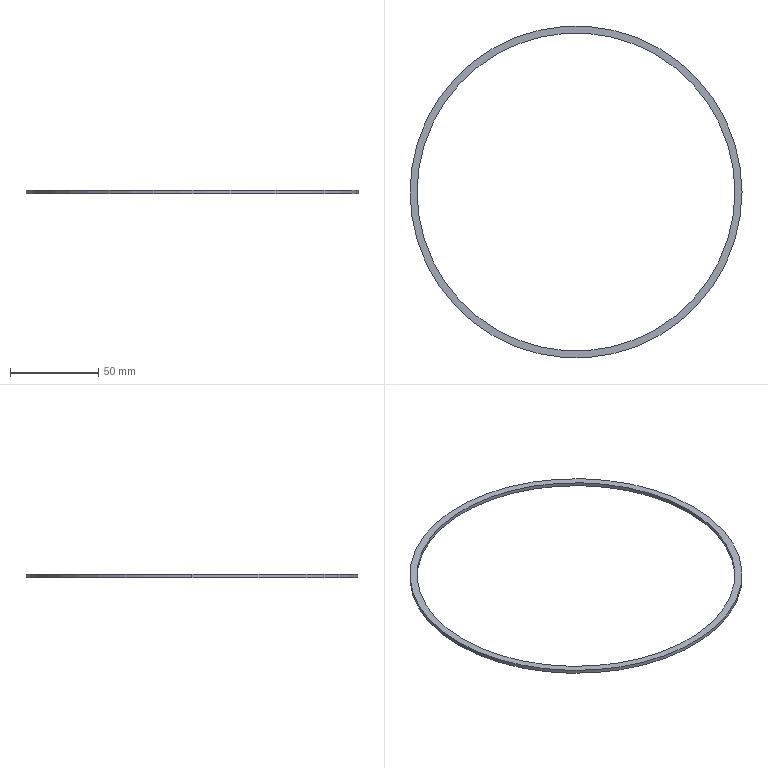Part | SolidWorks | features Extrusion 1 | 1 solid | 6 faces | box 188 x 188 x 2 mm | volume 4624 mm3 | cylinder 4 | plane 2 | commonest cylinder face diameters 180 x2 188 x2
STEP:
#1=CARTESIAN_POINT('',(-90.,0.,-1.));
#2=VERTEX_POINT('',#1);
#3=CARTESIAN_POINT('',(90.,0.,-1.));
#4=VERTEX_POINT('',#3);
#5=CARTESIAN_POINT('',(0.,0.,-1.));
#6=DIRECTION('',(0.,0.,1.));
#7=DIRECTION('',(1.,0.,0.));
#8=AXIS2_PLACEMENT_3D('',#5,#6,#7);
#9=CIRCLE('',#8,90.);
#10=EDGE_CURVE('',#2,#4,#9,.T.);
#11=ORIENTED_EDGE('',*,*,#10,.F.);
#12=CARTESIAN_POINT('',(-90.,0.,1.));
#13=VERTEX_POINT('',#12);
#14=CARTESIAN_POINT('',(-90.,0.,-1.));
#15=DIRECTION('',(0.,0.,1.));
#16=VECTOR('',#15,1000.);
#17=LINE('',#14,#16);
#18=EDGE_CURVE('',#2,#13,#17,.T.);
#19=ORIENTED_EDGE('',*,*,#18,.T.);
#20=CARTESIAN_POINT('',(90.,0.,1.));
#21=VERTEX_POINT('',#20);
#22=CARTESIAN_POINT('',(0.,0.,1.));
#23=DIRECTION('',(0.,0.,1.));
#24=DIRECTION('',(1.,0.,0.));
#25=AXIS2_PLACEMENT_3D('',#22,#23,#24);
#26=CIRCLE('',#25,90.);
#27=EDGE_CURVE('',#13,#21,#26,.T.);
#28=ORIENTED_EDGE('',*,*,#27,.T.);
#29=CARTESIAN_POINT('',(90.,0.,-1.));
#30=DIRECTION('',(0.,0.,1.));
#31=VECTOR('',#30,1000.);
#32=LINE('',#29,#31);
#33=EDGE_CURVE('',#4,#21,#32,.T.);
#34=ORIENTED_EDGE('',*,*,#33,.F.);
#35=EDGE_LOOP('',(#11,#19,#28,#34));
#36=FACE_OUTER_BOUND('',#35,.T.);
#37=CARTESIAN_POINT('',(0.,0.,-1.));
#38=DIRECTION('',(0.,0.,1.));
#39=DIRECTION('',(1.,0.,0.));
#40=AXIS2_PLACEMENT_3D('',#37,#38,#39);
#41=CYLINDRICAL_SURFACE('',#40,90.);
#42=ADVANCED_FACE('',(#36),#41,.F.);
#43=CARTESIAN_POINT('',(94.,0.,-1.));
#44=VERTEX_POINT('',#43);
#45=CARTESIAN_POINT('',(-94.,0.,-1.));
#46=VERTEX_POINT('',#45);
#47=CARTESIAN_POINT('',(0.,0.,-1.));
#48=DIRECTION('',(0.,0.,1.));
#49=DIRECTION('',(1.,0.,0.));
#50=AXIS2_PLACEMENT_3D('',#47,#48,#49);
#51=CIRCLE('',#50,94.);
#52=EDGE_CURVE('',#44,#46,#51,.T.);
#53=ORIENTED_EDGE('',*,*,#52,.T.);
#54=CARTESIAN_POINT('',(-94.,0.,1.));
#55=VERTEX_POINT('',#54);
#56=CARTESIAN_POINT('',(-94.,0.,-1.));
#57=DIRECTION('',(0.,0.,1.));
#58=VECTOR('',#57,1000.);
#59=LINE('',#56,#58);
#60=EDGE_CURVE('',#46,#55,#59,.T.);
#61=ORIENTED_EDGE('',*,*,#60,.T.);
#62=CARTESIAN_POINT('',(94.,0.,1.));
#63=VERTEX_POINT('',#62);
#64=CARTESIAN_POINT('',(0.,0.,1.));
#65=DIRECTION('',(0.,0.,1.));
#66=DIRECTION('',(1.,0.,0.));
#67=AXIS2_PLACEMENT_3D('',#64,#65,#66);
#68=CIRCLE('',#67,94.);
#69=EDGE_CURVE('',#63,#55,#68,.T.);
#70=ORIENTED_EDGE('',*,*,#69,.F.);
#71=CARTESIAN_POINT('',(94.,0.,-1.));
#72=DIRECTION('',(0.,0.,1.));
#73=VECTOR('',#72,1000.);
#74=LINE('',#71,#73);
#75=EDGE_CURVE('',#44,#63,#74,.T.);
#76=ORIENTED_EDGE('',*,*,#75,.F.);
#77=EDGE_LOOP('',(#53,#61,#70,#76));
#78=FACE_OUTER_BOUND('',#77,.T.);
#79=CARTESIAN_POINT('',(0.,0.,-1.));
#80=DIRECTION('',(0.,0.,1.));
#81=DIRECTION('',(1.,0.,0.));
#82=AXIS2_PLACEMENT_3D('',#79,#80,#81);
#83=CYLINDRICAL_SURFACE('',#82,94.);
#84=ADVANCED_FACE('',(#78),#83,.T.);
#85=ORIENTED_EDGE('',*,*,#60,.F.);
#86=CARTESIAN_POINT('',(0.,0.,-1.));
#87=DIRECTION('',(0.,0.,1.));
#88=DIRECTION('',(1.,0.,0.));
#89=AXIS2_PLACEMENT_3D('',#86,#87,#88);
#90=CIRCLE('',#89,94.);
#91=EDGE_CURVE('',#46,#44,#90,.T.);
#92=ORIENTED_EDGE('',*,*,#91,.T.);
#93=ORIENTED_EDGE('',*,*,#75,.T.);
#94=CARTESIAN_POINT('',(0.,0.,1.));
#95=DIRECTION('',(0.,0.,1.));
#96=DIRECTION('',(1.,0.,0.));
#97=AXIS2_PLACEMENT_3D('',#94,#95,#96);
#98=CIRCLE('',#97,94.);
#99=EDGE_CURVE('',#55,#63,#98,.T.);
#100=ORIENTED_EDGE('',*,*,#99,.F.);
#101=EDGE_LOOP('',(#85,#92,#93,#100));
#102=FACE_OUTER_BOUND('',#101,.T.);
#103=CARTESIAN_POINT('',(0.,0.,-1.));
#104=DIRECTION('',(0.,0.,1.));
#105=DIRECTION('',(1.,0.,0.));
#106=AXIS2_PLACEMENT_3D('',#103,#104,#105);
#107=CYLINDRICAL_SURFACE('',#106,94.);
#108=ADVANCED_FACE('',(#102),#107,.T.);
#109=CARTESIAN_POINT('',(0.,0.,-1.));
#110=DIRECTION('',(0.,0.,1.));
#111=DIRECTION('',(1.,0.,0.));
#112=AXIS2_PLACEMENT_3D('',#109,#110,#111);
#113=CIRCLE('',#112,90.);
#114=EDGE_CURVE('',#4,#2,#113,.T.);
#115=ORIENTED_EDGE('',*,*,#114,.T.);
#116=ORIENTED_EDGE('',*,*,#10,.T.);
#117=EDGE_LOOP('',(#115,#116));
#118=FACE_BOUND('',#117,.T.);
#119=ORIENTED_EDGE('',*,*,#52,.F.);
#120=ORIENTED_EDGE('',*,*,#91,.F.);
#121=EDGE_LOOP('',(#119,#120));
#122=FACE_OUTER_BOUND('',#121,.T.);
#123=CARTESIAN_POINT('',(0.,0.,-1.));
#124=DIRECTION('',(0.,0.,1.));
#125=DIRECTION('',(1.,0.,0.));
#126=AXIS2_PLACEMENT_3D('',#123,#124,#125);
#127=PLANE('',#126);
#128=ADVANCED_FACE('',(#118,#122),#127,.F.);
#129=CARTESIAN_POINT('',(0.,0.,1.));
#130=DIRECTION('',(0.,0.,1.));
#131=DIRECTION('',(1.,0.,0.));
#132=AXIS2_PLACEMENT_3D('',#129,#130,#131);
#133=CIRCLE('',#132,90.);
#134=EDGE_CURVE('',#21,#13,#133,.T.);
#135=ORIENTED_EDGE('',*,*,#134,.F.);
#136=ORIENTED_EDGE('',*,*,#27,.F.);
#137=EDGE_LOOP('',(#135,#136));
#138=FACE_BOUND('',#137,.T.);
#139=ORIENTED_EDGE('',*,*,#69,.T.);
#140=ORIENTED_EDGE('',*,*,#99,.T.);
#141=EDGE_LOOP('',(#139,#140));
#142=FACE_OUTER_BOUND('',#141,.T.);
#143=CARTESIAN_POINT('',(0.,0.,1.));
#144=DIRECTION('',(0.,0.,1.));
#145=DIRECTION('',(1.,0.,0.));
#146=AXIS2_PLACEMENT_3D('',#143,#144,#145);
#147=PLANE('',#146);
#148=ADVANCED_FACE('',(#138,#142),#147,.T.);
#149=ORIENTED_EDGE('',*,*,#18,.F.);
#150=ORIENTED_EDGE('',*,*,#114,.F.);
#151=ORIENTED_EDGE('',*,*,#33,.T.);
#152=ORIENTED_EDGE('',*,*,#134,.T.);
#153=EDGE_LOOP('',(#149,#150,#151,#152));
#154=FACE_OUTER_BOUND('',#153,.T.);
#155=CARTESIAN_POINT('',(0.,0.,-1.));
#156=DIRECTION('',(0.,0.,1.));
#157=DIRECTION('',(1.,0.,0.));
#158=AXIS2_PLACEMENT_3D('',#155,#156,#157);
#159=CYLINDRICAL_SURFACE('',#158,90.);
#160=ADVANCED_FACE('',(#154),#159,.F.);
#161=CLOSED_SHELL('',(#42,#84,#108,#128,#148,#160));
#162=MANIFOLD_SOLID_BREP('',#161);
#163=CARTESIAN_POINT('',(0.,0.,0.));
#164=DIRECTION('',(0.,0.,1.));
#165=DIRECTION('',(1.,0.,0.));
#166=AXIS2_PLACEMENT_3D('',#163,#164,#165);
#167=(LENGTH_UNIT()NAMED_UNIT(*)SI_UNIT(.MILLI.,.METRE.));
#168=UNCERTAINTY_MEASURE_WITH_UNIT(LENGTH_MEASURE(0.00001),#167,'','');
#169=(NAMED_UNIT(*)PLANE_ANGLE_UNIT()SI_UNIT($,.RADIAN.));
#170=(NAMED_UNIT(*)SI_UNIT($,.STERADIAN.)SOLID_ANGLE_UNIT());
#171=(GEOMETRIC_REPRESENTATION_CONTEXT(3)GLOBAL_UNCERTAINTY_ASSIGNED_CONTEXT((#168))GLOBAL_UNIT_ASSIGNED_CONTEXT((#167,#169,#170))REPRESENTATION_CONTEXT('',''));
#172=ADVANCED_BREP_SHAPE_REPRESENTATION('',(#162,#166),#171);